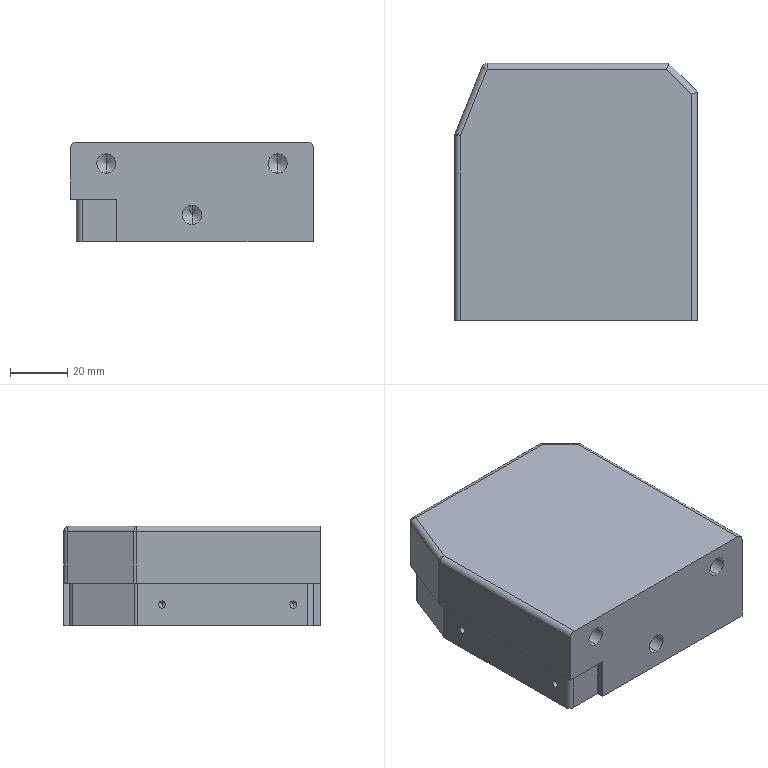Part | STEP file | Guide rail stopper 111 | 1 solid | 67 faces | box 85 x 90 x 35 mm | volume 251654 mm3 | cylinder 27 | plane 22 | cone 16 | sphere 2 | commonest cylinder face diameters 4 x11 2.5 x10 6.8 x6